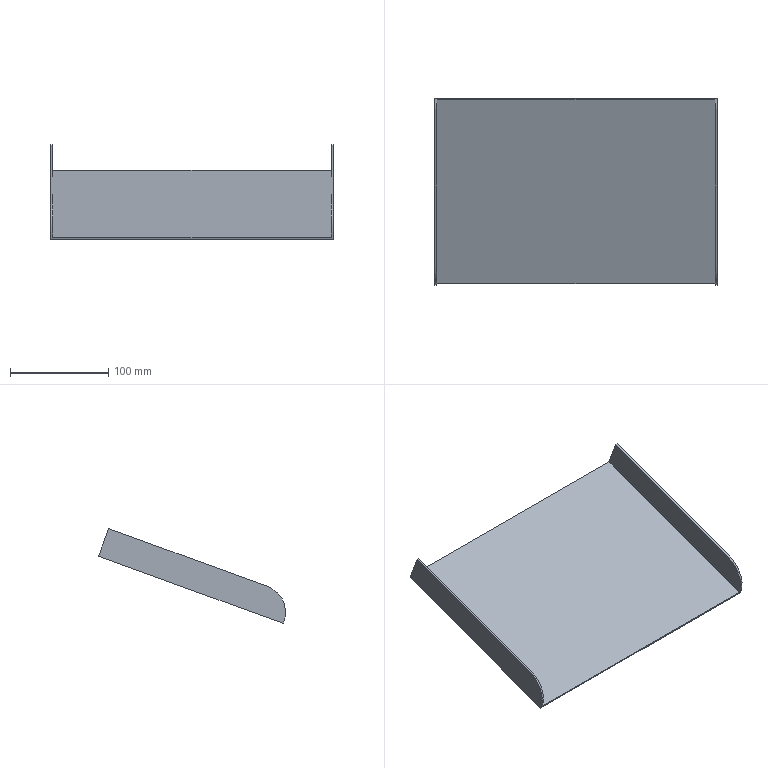Part | NX | features solid 2 | 1 solid | 12 faces | box 287.787 x 190.311 x 96.595 mm | volume 136842 mm3 | plane 10 | cylinder 2 | commonest cylinder face diameters 56 x2
STEP:
#1=CARTESIAN_POINT('',(702.,-997.939,-365.986));
#2=VERTEX_POINT('',#1);
#3=CARTESIAN_POINT('',(985.787,-997.939,-365.986));
#4=VERTEX_POINT('',#3);
#5=CARTESIAN_POINT('',(712.,-997.939,-365.986));
#6=DIRECTION('',(-1.,0.,0.));
#7=VECTOR('',#6,1000.);
#8=LINE('',#5,#7);
#9=EDGE_CURVE('',#2,#4,#8,.F.);
#10=ORIENTED_EDGE('',*,*,#9,.T.);
#11=CARTESIAN_POINT('',(985.787,-810.,-297.582));
#12=VERTEX_POINT('',#11);
#13=CARTESIAN_POINT('',(985.787,-838.191,-307.843));
#14=DIRECTION('',(0.,0.9397,0.342));
#15=VECTOR('',#14,1000.);
#16=LINE('',#13,#15);
#17=EDGE_CURVE('',#4,#12,#16,.T.);
#18=ORIENTED_EDGE('',*,*,#17,.T.);
#19=CARTESIAN_POINT('',(702.,-810.,-297.582));
#20=VERTEX_POINT('',#19);
#21=CARTESIAN_POINT('',(712.,-810.,-297.582));
#22=DIRECTION('',(1.,0.,0.));
#23=VECTOR('',#22,1000.);
#24=LINE('',#21,#23);
#25=EDGE_CURVE('',#20,#12,#24,.T.);
#26=ORIENTED_EDGE('',*,*,#25,.F.);
#27=CARTESIAN_POINT('',(702.,-838.191,-307.843));
#28=DIRECTION('',(0.,0.9397,0.342));
#29=VECTOR('',#28,1000.);
#30=LINE('',#27,#29);
#31=EDGE_CURVE('',#2,#20,#30,.T.);
#32=ORIENTED_EDGE('',*,*,#31,.F.);
#33=EDGE_LOOP('',(#10,#18,#26,#32));
#34=FACE_BOUND('',#33,.T.);
#35=CARTESIAN_POINT('',(712.,-838.191,-307.843));
#36=DIRECTION('',(0.,0.342,-0.9397));
#37=DIRECTION('',(-1.,0.,0.));
#38=AXIS2_PLACEMENT_3D('',#35,#36,#37);
#39=PLANE('',#38);
#40=ADVANCED_FACE('',(#34),#39,.F.);
#41=ORIENTED_EDGE('',*,*,#25,.T.);
#42=CARTESIAN_POINT('',(985.787,-819.577,-271.271));
#43=VERTEX_POINT('',#42);
#44=CARTESIAN_POINT('',(985.787,-809.316,-299.462));
#45=DIRECTION('',(0.,-0.342,0.9397));
#46=VECTOR('',#45,1000.);
#47=LINE('',#44,#46);
#48=EDGE_CURVE('',#12,#43,#47,.T.);
#49=ORIENTED_EDGE('',*,*,#48,.T.);
#50=CARTESIAN_POINT('',(987.787,-819.577,-271.271));
#51=VERTEX_POINT('',#50);
#52=CARTESIAN_POINT('',(987.787,-819.577,-271.271));
#53=DIRECTION('',(1.,0.,0.));
#54=VECTOR('',#53,1000.);
#55=LINE('',#52,#54);
#56=EDGE_CURVE('',#51,#43,#55,.F.);
#57=ORIENTED_EDGE('',*,*,#56,.F.);
#58=CARTESIAN_POINT('',(987.787,-809.316,-299.462));
#59=VERTEX_POINT('',#58);
#60=CARTESIAN_POINT('',(987.787,-809.316,-299.462));
#61=DIRECTION('',(0.,-0.342,0.9397));
#62=VECTOR('',#61,1000.);
#63=LINE('',#60,#62);
#64=EDGE_CURVE('',#59,#51,#63,.T.);
#65=ORIENTED_EDGE('',*,*,#64,.F.);
#66=CARTESIAN_POINT('',(700.,-809.316,-299.462));
#67=VERTEX_POINT('',#66);
#68=CARTESIAN_POINT('',(712.,-809.316,-299.462));
#69=DIRECTION('',(1.,0.,0.));
#70=VECTOR('',#69,1000.);
#71=LINE('',#68,#70);
#72=EDGE_CURVE('',#67,#59,#71,.T.);
#73=ORIENTED_EDGE('',*,*,#72,.F.);
#74=CARTESIAN_POINT('',(700.,-819.577,-271.271));
#75=VERTEX_POINT('',#74);
#76=CARTESIAN_POINT('',(700.,-809.316,-299.462));
#77=DIRECTION('',(0.,0.342,-0.9397));
#78=VECTOR('',#77,1000.);
#79=LINE('',#76,#78);
#80=EDGE_CURVE('',#67,#75,#79,.F.);
#81=ORIENTED_EDGE('',*,*,#80,.T.);
#82=CARTESIAN_POINT('',(702.,-819.577,-271.271));
#83=VERTEX_POINT('',#82);
#84=CARTESIAN_POINT('',(700.,-819.577,-271.271));
#85=DIRECTION('',(1.,0.,0.));
#86=VECTOR('',#85,1000.);
#87=LINE('',#84,#86);
#88=EDGE_CURVE('',#75,#83,#87,.T.);
#89=ORIENTED_EDGE('',*,*,#88,.T.);
#90=CARTESIAN_POINT('',(702.,-809.316,-299.462));
#91=DIRECTION('',(0.,-0.342,0.9397));
#92=VECTOR('',#91,1000.);
#93=LINE('',#90,#92);
#94=EDGE_CURVE('',#20,#83,#93,.T.);
#95=ORIENTED_EDGE('',*,*,#94,.F.);
#96=EDGE_LOOP('',(#41,#49,#57,#65,#73,#81,#89,#95));
#97=FACE_BOUND('',#96,.T.);
#98=CARTESIAN_POINT('',(712.,-809.316,-299.462));
#99=DIRECTION('',(0.,0.9397,0.342));
#100=DIRECTION('',(1.,0.,0.));
#101=AXIS2_PLACEMENT_3D('',#98,#99,#100);
#102=PLANE('',#101);
#103=ADVANCED_FACE('',(#97),#102,.T.);
#104=ORIENTED_EDGE('',*,*,#80,.F.);
#105=CARTESIAN_POINT('',(700.,-997.254,-367.866));
#106=VERTEX_POINT('',#105);
#107=CARTESIAN_POINT('',(700.,-837.507,-309.722));
#108=DIRECTION('',(0.,0.9397,0.342));
#109=VECTOR('',#108,1000.);
#110=LINE('',#107,#109);
#111=EDGE_CURVE('',#67,#106,#110,.F.);
#112=ORIENTED_EDGE('',*,*,#111,.T.);
#113=CARTESIAN_POINT('',(700.,-997.939,-365.986));
#114=VERTEX_POINT('',#113);
#115=CARTESIAN_POINT('',(700.,-997.254,-367.866));
#116=DIRECTION('',(0.,-0.342,0.9397));
#117=VECTOR('',#116,1000.);
#118=LINE('',#115,#117);
#119=EDGE_CURVE('',#106,#114,#118,.T.);
#120=ORIENTED_EDGE('',*,*,#119,.T.);
#121=CARTESIAN_POINT('',(700.,-981.204,-330.098));
#122=VERTEX_POINT('',#121);
#123=CARTESIAN_POINT('',(700.,-971.627,-356.41));
#124=DIRECTION('',(-1.,0.,0.));
#125=DIRECTION('',(0.,0.,1.));
#126=AXIS2_PLACEMENT_3D('',#123,#124,#125);
#127=CIRCLE('',#126,28.);
#128=EDGE_CURVE('',#114,#122,#127,.T.);
#129=ORIENTED_EDGE('',*,*,#128,.T.);
#130=CARTESIAN_POINT('',(700.,-819.577,-271.271));
#131=DIRECTION('',(0.,-0.9397,-0.342));
#132=VECTOR('',#131,1000.);
#133=LINE('',#130,#132);
#134=EDGE_CURVE('',#75,#122,#133,.T.);
#135=ORIENTED_EDGE('',*,*,#134,.F.);
#136=EDGE_LOOP('',(#104,#112,#120,#129,#135));
#137=FACE_BOUND('',#136,.T.);
#138=CARTESIAN_POINT('',(700.,-837.507,-309.722));
#139=DIRECTION('',(1.,0.,0.));
#140=DIRECTION('',(0.,-0.9397,-0.342));
#141=AXIS2_PLACEMENT_3D('',#138,#139,#140);
#142=PLANE('',#141);
#143=ADVANCED_FACE('',(#137),#142,.F.);
#144=CARTESIAN_POINT('',(987.787,-997.254,-367.866));
#145=VERTEX_POINT('',#144);
#146=CARTESIAN_POINT('',(712.,-997.254,-367.866));
#147=DIRECTION('',(1.,0.,0.));
#148=VECTOR('',#147,1000.);
#149=LINE('',#146,#148);
#150=EDGE_CURVE('',#106,#145,#149,.T.);
#151=ORIENTED_EDGE('',*,*,#150,.T.);
#152=CARTESIAN_POINT('',(987.787,-997.939,-365.986));
#153=VERTEX_POINT('',#152);
#154=CARTESIAN_POINT('',(987.787,-997.254,-367.866));
#155=DIRECTION('',(0.,0.342,-0.9397));
#156=VECTOR('',#155,1000.);
#157=LINE('',#154,#156);
#158=EDGE_CURVE('',#145,#153,#157,.F.);
#159=ORIENTED_EDGE('',*,*,#158,.T.);
#160=CARTESIAN_POINT('',(987.787,-997.939,-365.986));
#161=DIRECTION('',(-1.,0.,0.));
#162=VECTOR('',#161,1000.);
#163=LINE('',#160,#162);
#164=EDGE_CURVE('',#153,#4,#163,.T.);
#165=ORIENTED_EDGE('',*,*,#164,.T.);
#166=ORIENTED_EDGE('',*,*,#9,.F.);
#167=CARTESIAN_POINT('',(712.,-997.939,-365.986));
#168=DIRECTION('',(-1.,0.,0.));
#169=VECTOR('',#168,1000.);
#170=LINE('',#167,#169);
#171=EDGE_CURVE('',#114,#2,#170,.F.);
#172=ORIENTED_EDGE('',*,*,#171,.F.);
#173=ORIENTED_EDGE('',*,*,#119,.F.);
#174=EDGE_LOOP('',(#151,#159,#165,#166,#172,#173));
#175=FACE_BOUND('',#174,.T.);
#176=CARTESIAN_POINT('',(712.,-997.254,-367.866));
#177=DIRECTION('',(0.,0.9397,0.342));
#178=DIRECTION('',(1.,0.,0.));
#179=AXIS2_PLACEMENT_3D('',#176,#177,#178);
#180=PLANE('',#179);
#181=ADVANCED_FACE('',(#175),#180,.F.);
#182=CARTESIAN_POINT('',(987.787,-837.507,-309.722));
#183=DIRECTION('',(0.,-0.9397,-0.342));
#184=VECTOR('',#183,1000.);
#185=LINE('',#182,#184);
#186=EDGE_CURVE('',#59,#145,#185,.T.);
#187=ORIENTED_EDGE('',*,*,#186,.F.);
#188=ORIENTED_EDGE('',*,*,#64,.T.);
#189=CARTESIAN_POINT('',(987.787,-981.204,-330.098));
#190=VERTEX_POINT('',#189);
#191=CARTESIAN_POINT('',(987.787,-819.577,-271.271));
#192=DIRECTION('',(0.,-0.9397,-0.342));
#193=VECTOR('',#192,1000.);
#194=LINE('',#191,#193);
#195=EDGE_CURVE('',#51,#190,#194,.T.);
#196=ORIENTED_EDGE('',*,*,#195,.T.);
#197=CARTESIAN_POINT('',(987.787,-971.627,-356.41));
#198=DIRECTION('',(-1.,0.,0.));
#199=DIRECTION('',(0.,0.,1.));
#200=AXIS2_PLACEMENT_3D('',#197,#198,#199);
#201=CIRCLE('',#200,28.);
#202=EDGE_CURVE('',#190,#153,#201,.F.);
#203=ORIENTED_EDGE('',*,*,#202,.T.);
#204=ORIENTED_EDGE('',*,*,#158,.F.);
#205=EDGE_LOOP('',(#187,#188,#196,#203,#204));
#206=FACE_BOUND('',#205,.T.);
#207=CARTESIAN_POINT('',(987.787,-837.507,-309.722));
#208=DIRECTION('',(1.,0.,0.));
#209=DIRECTION('',(0.,-0.9397,-0.342));
#210=AXIS2_PLACEMENT_3D('',#207,#208,#209);
#211=PLANE('',#210);
#212=ADVANCED_FACE('',(#206),#211,.T.);
#213=ORIENTED_EDGE('',*,*,#72,.T.);
#214=ORIENTED_EDGE('',*,*,#186,.T.);
#215=ORIENTED_EDGE('',*,*,#150,.F.);
#216=ORIENTED_EDGE('',*,*,#111,.F.);
#217=EDGE_LOOP('',(#213,#214,#215,#216));
#218=FACE_BOUND('',#217,.T.);
#219=CARTESIAN_POINT('',(712.,-837.507,-309.722));
#220=DIRECTION('',(0.,0.342,-0.9397));
#221=DIRECTION('',(-1.,0.,0.));
#222=AXIS2_PLACEMENT_3D('',#219,#220,#221);
#223=PLANE('',#222);
#224=ADVANCED_FACE('',(#218),#223,.T.);
#225=CARTESIAN_POINT('',(702.,-981.204,-330.098));
#226=VERTEX_POINT('',#225);
#227=CARTESIAN_POINT('',(702.,-971.627,-356.41));
#228=DIRECTION('',(-1.,0.,0.));
#229=DIRECTION('',(0.,0.,1.));
#230=AXIS2_PLACEMENT_3D('',#227,#228,#229);
#231=CIRCLE('',#230,28.);
#232=EDGE_CURVE('',#226,#2,#231,.F.);
#233=ORIENTED_EDGE('',*,*,#232,.T.);
#234=ORIENTED_EDGE('',*,*,#31,.T.);
#235=ORIENTED_EDGE('',*,*,#94,.T.);
#236=CARTESIAN_POINT('',(702.,-819.577,-271.271));
#237=DIRECTION('',(0.,-0.9397,-0.342));
#238=VECTOR('',#237,1000.);
#239=LINE('',#236,#238);
#240=EDGE_CURVE('',#83,#226,#239,.T.);
#241=ORIENTED_EDGE('',*,*,#240,.T.);
#242=EDGE_LOOP('',(#233,#234,#235,#241));
#243=FACE_BOUND('',#242,.T.);
#244=CARTESIAN_POINT('',(702.,-809.316,-299.462));
#245=DIRECTION('',(-1.,0.,0.));
#246=DIRECTION('',(0.,0.,1.));
#247=AXIS2_PLACEMENT_3D('',#244,#245,#246);
#248=PLANE('',#247);
#249=ADVANCED_FACE('',(#243),#248,.F.);
#250=ORIENTED_EDGE('',*,*,#134,.T.);
#251=CARTESIAN_POINT('',(700.,-981.204,-330.098));
#252=DIRECTION('',(1.,0.,0.));
#253=VECTOR('',#252,1000.);
#254=LINE('',#251,#253);
#255=EDGE_CURVE('',#122,#226,#254,.T.);
#256=ORIENTED_EDGE('',*,*,#255,.T.);
#257=ORIENTED_EDGE('',*,*,#240,.F.);
#258=ORIENTED_EDGE('',*,*,#88,.F.);
#259=EDGE_LOOP('',(#250,#256,#257,#258));
#260=FACE_BOUND('',#259,.T.);
#261=CARTESIAN_POINT('',(700.,-819.577,-271.271));
#262=DIRECTION('',(0.,0.342,-0.9397));
#263=DIRECTION('',(0.,-0.9397,-0.342));
#264=AXIS2_PLACEMENT_3D('',#261,#262,#263);
#265=PLANE('',#264);
#266=ADVANCED_FACE('',(#260),#265,.F.);
#267=ORIENTED_EDGE('',*,*,#128,.F.);
#268=ORIENTED_EDGE('',*,*,#171,.T.);
#269=ORIENTED_EDGE('',*,*,#232,.F.);
#270=ORIENTED_EDGE('',*,*,#255,.F.);
#271=EDGE_LOOP('',(#267,#268,#269,#270));
#272=FACE_BOUND('',#271,.T.);
#273=CARTESIAN_POINT('',(700.,-971.627,-356.41));
#274=DIRECTION('',(-1.,0.,0.));
#275=DIRECTION('',(0.,0.,1.));
#276=AXIS2_PLACEMENT_3D('',#273,#274,#275);
#277=CYLINDRICAL_SURFACE('',#276,28.);
#278=ADVANCED_FACE('',(#272),#277,.T.);
#279=ORIENTED_EDGE('',*,*,#17,.F.);
#280=CARTESIAN_POINT('',(985.787,-981.204,-330.098));
#281=VERTEX_POINT('',#280);
#282=CARTESIAN_POINT('',(985.787,-971.627,-356.41));
#283=DIRECTION('',(-1.,0.,0.));
#284=DIRECTION('',(0.,0.,1.));
#285=AXIS2_PLACEMENT_3D('',#282,#283,#284);
#286=CIRCLE('',#285,28.);
#287=EDGE_CURVE('',#4,#281,#286,.T.);
#288=ORIENTED_EDGE('',*,*,#287,.T.);
#289=CARTESIAN_POINT('',(985.787,-819.577,-271.271));
#290=DIRECTION('',(0.,-0.9397,-0.342));
#291=VECTOR('',#290,1000.);
#292=LINE('',#289,#291);
#293=EDGE_CURVE('',#43,#281,#292,.T.);
#294=ORIENTED_EDGE('',*,*,#293,.F.);
#295=ORIENTED_EDGE('',*,*,#48,.F.);
#296=EDGE_LOOP('',(#279,#288,#294,#295));
#297=FACE_BOUND('',#296,.T.);
#298=CARTESIAN_POINT('',(985.787,-809.316,-299.462));
#299=DIRECTION('',(-1.,0.,0.));
#300=DIRECTION('',(0.,0.,1.));
#301=AXIS2_PLACEMENT_3D('',#298,#299,#300);
#302=PLANE('',#301);
#303=ADVANCED_FACE('',(#297),#302,.T.);
#304=ORIENTED_EDGE('',*,*,#293,.T.);
#305=CARTESIAN_POINT('',(987.787,-981.204,-330.098));
#306=DIRECTION('',(1.,0.,0.));
#307=VECTOR('',#306,1000.);
#308=LINE('',#305,#307);
#309=EDGE_CURVE('',#281,#190,#308,.T.);
#310=ORIENTED_EDGE('',*,*,#309,.T.);
#311=ORIENTED_EDGE('',*,*,#195,.F.);
#312=ORIENTED_EDGE('',*,*,#56,.T.);
#313=EDGE_LOOP('',(#304,#310,#311,#312));
#314=FACE_BOUND('',#313,.T.);
#315=CARTESIAN_POINT('',(987.787,-819.577,-271.271));
#316=DIRECTION('',(0.,0.342,-0.9397));
#317=DIRECTION('',(0.,-0.9397,-0.342));
#318=AXIS2_PLACEMENT_3D('',#315,#316,#317);
#319=PLANE('',#318);
#320=ADVANCED_FACE('',(#314),#319,.F.);
#321=ORIENTED_EDGE('',*,*,#202,.F.);
#322=ORIENTED_EDGE('',*,*,#309,.F.);
#323=ORIENTED_EDGE('',*,*,#287,.F.);
#324=ORIENTED_EDGE('',*,*,#164,.F.);
#325=EDGE_LOOP('',(#321,#322,#323,#324));
#326=FACE_BOUND('',#325,.T.);
#327=CARTESIAN_POINT('',(987.787,-971.627,-356.41));
#328=DIRECTION('',(1.,0.,0.));
#329=DIRECTION('',(0.,0.,-1.));
#330=AXIS2_PLACEMENT_3D('',#327,#328,#329);
#331=CYLINDRICAL_SURFACE('',#330,28.);
#332=ADVANCED_FACE('',(#326),#331,.T.);
#333=CLOSED_SHELL('',(#40,#103,#143,#181,#212,#224,#249,#266,#278,#303,#320,#332));
#334=MANIFOLD_SOLID_BREP('',#333);
#335=(LENGTH_UNIT()NAMED_UNIT(*)SI_UNIT(.MILLI.,.METRE.));
#336=UNCERTAINTY_MEASURE_WITH_UNIT(LENGTH_MEASURE(0.00001),#335,'','');
#337=(NAMED_UNIT(*)PLANE_ANGLE_UNIT()SI_UNIT($,.RADIAN.));
#338=(NAMED_UNIT(*)SI_UNIT($,.STERADIAN.)SOLID_ANGLE_UNIT());
#339=(GEOMETRIC_REPRESENTATION_CONTEXT(3)GLOBAL_UNCERTAINTY_ASSIGNED_CONTEXT((#336))GLOBAL_UNIT_ASSIGNED_CONTEXT((#335,#337,#338))REPRESENTATION_CONTEXT('',''));
#340=ADVANCED_BREP_SHAPE_REPRESENTATION('',(#334),#339);